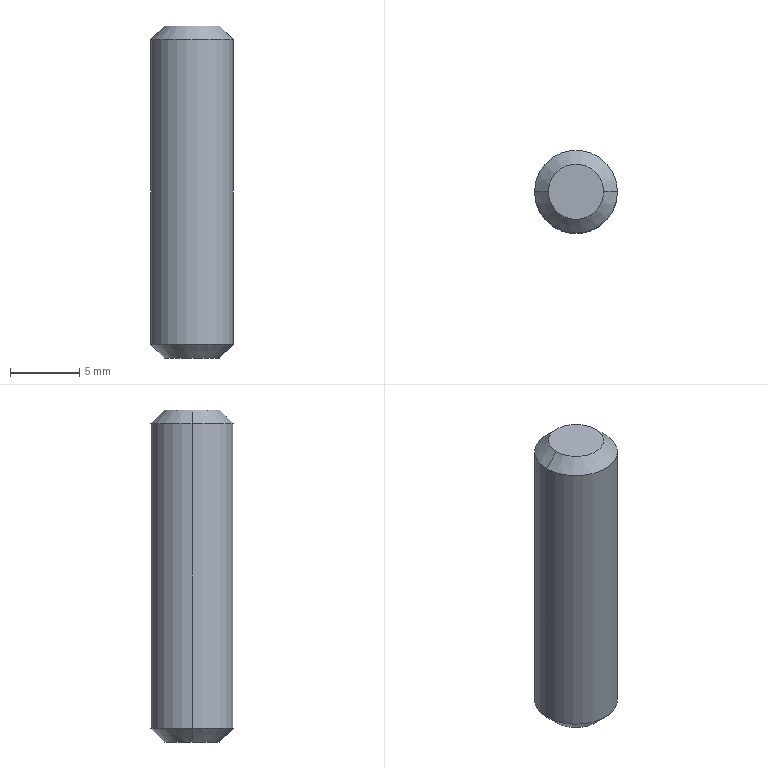Part | SolidWorks | features Chamfer 1, Extrusion 1 | 1 solid | 8 faces | box 6 x 6 x 24 mm | volume 661.829 mm3 | cone 4 | cylinder 2 | plane 2 | commonest cylinder face diameters 6 x2
STEP:
#1=CARTESIAN_POINT('',(2.,0.,24.));
#2=VERTEX_POINT('',#1);
#3=CARTESIAN_POINT('',(-2.,0.,24.));
#4=VERTEX_POINT('',#3);
#5=CARTESIAN_POINT('',(0.,0.,24.));
#6=DIRECTION('',(0.,0.,1.));
#7=DIRECTION('',(1.,0.,0.));
#8=AXIS2_PLACEMENT_3D('',#5,#6,#7);
#9=CIRCLE('',#8,2.);
#10=EDGE_CURVE('',#2,#4,#9,.T.);
#11=ORIENTED_EDGE('',*,*,#10,.F.);
#12=CARTESIAN_POINT('',(3.,0.,23.));
#13=VERTEX_POINT('',#12);
#14=CARTESIAN_POINT('',(2.,0.,24.));
#15=DIRECTION('',(0.7071,0.,-0.7071));
#16=VECTOR('',#15,1000.);
#17=LINE('',#14,#16);
#18=EDGE_CURVE('',#2,#13,#17,.T.);
#19=ORIENTED_EDGE('',*,*,#18,.T.);
#20=CARTESIAN_POINT('',(-3.,0.,23.));
#21=VERTEX_POINT('',#20);
#22=CARTESIAN_POINT('',(0.,0.,23.));
#23=DIRECTION('',(0.,0.,-1.));
#24=DIRECTION('',(1.,0.,0.));
#25=AXIS2_PLACEMENT_3D('',#22,#23,#24);
#26=CIRCLE('',#25,3.);
#27=EDGE_CURVE('',#21,#13,#26,.T.);
#28=ORIENTED_EDGE('',*,*,#27,.F.);
#29=CARTESIAN_POINT('',(-2.,0.,24.));
#30=DIRECTION('',(-0.7071,0.,-0.7071));
#31=VECTOR('',#30,1000.);
#32=LINE('',#29,#31);
#33=EDGE_CURVE('',#4,#21,#32,.T.);
#34=ORIENTED_EDGE('',*,*,#33,.F.);
#35=EDGE_LOOP('',(#11,#19,#28,#34));
#36=FACE_OUTER_BOUND('',#35,.T.);
#37=CARTESIAN_POINT('',(0.,0.,24.));
#38=DIRECTION('',(0.,0.,-1.));
#39=DIRECTION('',(-1.,0.,0.));
#40=AXIS2_PLACEMENT_3D('',#37,#38,#39);
#41=CONICAL_SURFACE('',#40,2.,0.7854);
#42=ADVANCED_FACE('',(#36),#41,.T.);
#43=CARTESIAN_POINT('',(-2.,0.,0.));
#44=VERTEX_POINT('',#43);
#45=CARTESIAN_POINT('',(2.,0.,0.));
#46=VERTEX_POINT('',#45);
#47=CARTESIAN_POINT('',(0.,0.,0.));
#48=DIRECTION('',(0.,0.,-1.));
#49=DIRECTION('',(1.,0.,0.));
#50=AXIS2_PLACEMENT_3D('',#47,#48,#49);
#51=CIRCLE('',#50,2.);
#52=EDGE_CURVE('',#44,#46,#51,.T.);
#53=ORIENTED_EDGE('',*,*,#52,.F.);
#54=CARTESIAN_POINT('',(-3.,0.,1.));
#55=VERTEX_POINT('',#54);
#56=CARTESIAN_POINT('',(-3.,0.,1.));
#57=DIRECTION('',(-0.7071,0.,0.7071));
#58=VECTOR('',#57,1000.);
#59=LINE('',#56,#58);
#60=EDGE_CURVE('',#44,#55,#59,.T.);
#61=ORIENTED_EDGE('',*,*,#60,.T.);
#62=CARTESIAN_POINT('',(3.,0.,1.));
#63=VERTEX_POINT('',#62);
#64=CARTESIAN_POINT('',(0.,0.,1.));
#65=DIRECTION('',(0.,0.,1.));
#66=DIRECTION('',(1.,0.,0.));
#67=AXIS2_PLACEMENT_3D('',#64,#65,#66);
#68=CIRCLE('',#67,3.);
#69=EDGE_CURVE('',#63,#55,#68,.T.);
#70=ORIENTED_EDGE('',*,*,#69,.F.);
#71=CARTESIAN_POINT('',(3.,0.,1.));
#72=DIRECTION('',(0.7071,0.,0.7071));
#73=VECTOR('',#72,1000.);
#74=LINE('',#71,#73);
#75=EDGE_CURVE('',#46,#63,#74,.T.);
#76=ORIENTED_EDGE('',*,*,#75,.F.);
#77=EDGE_LOOP('',(#53,#61,#70,#76));
#78=FACE_OUTER_BOUND('',#77,.T.);
#79=CARTESIAN_POINT('',(0.,0.,1.));
#80=DIRECTION('',(0.,0.,1.));
#81=DIRECTION('',(1.,0.,0.));
#82=AXIS2_PLACEMENT_3D('',#79,#80,#81);
#83=CONICAL_SURFACE('',#82,3.,0.7854);
#84=ADVANCED_FACE('',(#78),#83,.T.);
#85=ORIENTED_EDGE('',*,*,#27,.T.);
#86=CARTESIAN_POINT('',(3.,0.,24.));
#87=DIRECTION('',(0.,0.,-1.));
#88=VECTOR('',#87,1000.);
#89=LINE('',#86,#88);
#90=EDGE_CURVE('',#13,#63,#89,.T.);
#91=ORIENTED_EDGE('',*,*,#90,.T.);
#92=ORIENTED_EDGE('',*,*,#69,.T.);
#93=CARTESIAN_POINT('',(-3.,0.,24.));
#94=DIRECTION('',(0.,0.,-1.));
#95=VECTOR('',#94,1000.);
#96=LINE('',#93,#95);
#97=EDGE_CURVE('',#21,#55,#96,.T.);
#98=ORIENTED_EDGE('',*,*,#97,.F.);
#99=EDGE_LOOP('',(#85,#91,#92,#98));
#100=FACE_OUTER_BOUND('',#99,.T.);
#101=CARTESIAN_POINT('',(0.,0.,24.));
#102=DIRECTION('',(0.,0.,-1.));
#103=DIRECTION('',(-1.,0.,0.));
#104=AXIS2_PLACEMENT_3D('',#101,#102,#103);
#105=CYLINDRICAL_SURFACE('',#104,3.);
#106=ADVANCED_FACE('',(#100),#105,.T.);
#107=ORIENTED_EDGE('',*,*,#90,.F.);
#108=CARTESIAN_POINT('',(0.,0.,23.));
#109=DIRECTION('',(0.,0.,-1.));
#110=DIRECTION('',(1.,0.,0.));
#111=AXIS2_PLACEMENT_3D('',#108,#109,#110);
#112=CIRCLE('',#111,3.);
#113=EDGE_CURVE('',#13,#21,#112,.T.);
#114=ORIENTED_EDGE('',*,*,#113,.T.);
#115=ORIENTED_EDGE('',*,*,#97,.T.);
#116=CARTESIAN_POINT('',(0.,0.,1.));
#117=DIRECTION('',(0.,0.,1.));
#118=DIRECTION('',(1.,0.,0.));
#119=AXIS2_PLACEMENT_3D('',#116,#117,#118);
#120=CIRCLE('',#119,3.);
#121=EDGE_CURVE('',#55,#63,#120,.T.);
#122=ORIENTED_EDGE('',*,*,#121,.T.);
#123=EDGE_LOOP('',(#107,#114,#115,#122));
#124=FACE_OUTER_BOUND('',#123,.T.);
#125=CARTESIAN_POINT('',(0.,0.,24.));
#126=DIRECTION('',(0.,0.,-1.));
#127=DIRECTION('',(-1.,0.,0.));
#128=AXIS2_PLACEMENT_3D('',#125,#126,#127);
#129=CYLINDRICAL_SURFACE('',#128,3.);
#130=ADVANCED_FACE('',(#124),#129,.T.);
#131=CARTESIAN_POINT('',(0.,0.,24.));
#132=DIRECTION('',(0.,0.,1.));
#133=DIRECTION('',(1.,0.,0.));
#134=AXIS2_PLACEMENT_3D('',#131,#132,#133);
#135=CIRCLE('',#134,2.);
#136=EDGE_CURVE('',#4,#2,#135,.T.);
#137=ORIENTED_EDGE('',*,*,#136,.T.);
#138=ORIENTED_EDGE('',*,*,#10,.T.);
#139=EDGE_LOOP('',(#137,#138));
#140=FACE_OUTER_BOUND('',#139,.T.);
#141=CARTESIAN_POINT('',(0.,0.,24.));
#142=DIRECTION('',(0.,0.,1.));
#143=DIRECTION('',(1.,0.,0.));
#144=AXIS2_PLACEMENT_3D('',#141,#142,#143);
#145=PLANE('',#144);
#146=ADVANCED_FACE('',(#140),#145,.T.);
#147=CARTESIAN_POINT('',(0.,0.,0.));
#148=DIRECTION('',(0.,0.,-1.));
#149=DIRECTION('',(1.,0.,0.));
#150=AXIS2_PLACEMENT_3D('',#147,#148,#149);
#151=CIRCLE('',#150,2.);
#152=EDGE_CURVE('',#46,#44,#151,.T.);
#153=ORIENTED_EDGE('',*,*,#152,.T.);
#154=ORIENTED_EDGE('',*,*,#52,.T.);
#155=EDGE_LOOP('',(#153,#154));
#156=FACE_OUTER_BOUND('',#155,.T.);
#157=CARTESIAN_POINT('',(0.,0.,0.));
#158=DIRECTION('',(0.,0.,1.));
#159=DIRECTION('',(1.,0.,0.));
#160=AXIS2_PLACEMENT_3D('',#157,#158,#159);
#161=PLANE('',#160);
#162=ADVANCED_FACE('',(#156),#161,.F.);
#163=ORIENTED_EDGE('',*,*,#60,.F.);
#164=ORIENTED_EDGE('',*,*,#152,.F.);
#165=ORIENTED_EDGE('',*,*,#75,.T.);
#166=ORIENTED_EDGE('',*,*,#121,.F.);
#167=EDGE_LOOP('',(#163,#164,#165,#166));
#168=FACE_OUTER_BOUND('',#167,.T.);
#169=CARTESIAN_POINT('',(0.,0.,1.));
#170=DIRECTION('',(0.,0.,1.));
#171=DIRECTION('',(1.,0.,0.));
#172=AXIS2_PLACEMENT_3D('',#169,#170,#171);
#173=CONICAL_SURFACE('',#172,3.,0.7854);
#174=ADVANCED_FACE('',(#168),#173,.T.);
#175=ORIENTED_EDGE('',*,*,#18,.F.);
#176=ORIENTED_EDGE('',*,*,#136,.F.);
#177=ORIENTED_EDGE('',*,*,#33,.T.);
#178=ORIENTED_EDGE('',*,*,#113,.F.);
#179=EDGE_LOOP('',(#175,#176,#177,#178));
#180=FACE_OUTER_BOUND('',#179,.T.);
#181=CARTESIAN_POINT('',(0.,0.,24.));
#182=DIRECTION('',(0.,0.,-1.));
#183=DIRECTION('',(-1.,0.,0.));
#184=AXIS2_PLACEMENT_3D('',#181,#182,#183);
#185=CONICAL_SURFACE('',#184,2.,0.7854);
#186=ADVANCED_FACE('',(#180),#185,.T.);
#187=CLOSED_SHELL('',(#42,#84,#106,#130,#146,#162,#174,#186));
#188=MANIFOLD_SOLID_BREP('',#187);
#189=CARTESIAN_POINT('',(0.,0.,0.));
#190=DIRECTION('',(0.,0.,1.));
#191=DIRECTION('',(1.,0.,0.));
#192=AXIS2_PLACEMENT_3D('',#189,#190,#191);
#193=(LENGTH_UNIT()NAMED_UNIT(*)SI_UNIT(.MILLI.,.METRE.));
#194=UNCERTAINTY_MEASURE_WITH_UNIT(LENGTH_MEASURE(0.00001),#193,'','');
#195=(NAMED_UNIT(*)PLANE_ANGLE_UNIT()SI_UNIT($,.RADIAN.));
#196=(NAMED_UNIT(*)SI_UNIT($,.STERADIAN.)SOLID_ANGLE_UNIT());
#197=(GEOMETRIC_REPRESENTATION_CONTEXT(3)GLOBAL_UNCERTAINTY_ASSIGNED_CONTEXT((#194))GLOBAL_UNIT_ASSIGNED_CONTEXT((#193,#195,#196))REPRESENTATION_CONTEXT('',''));
#198=ADVANCED_BREP_SHAPE_REPRESENTATION('',(#188,#192),#197);